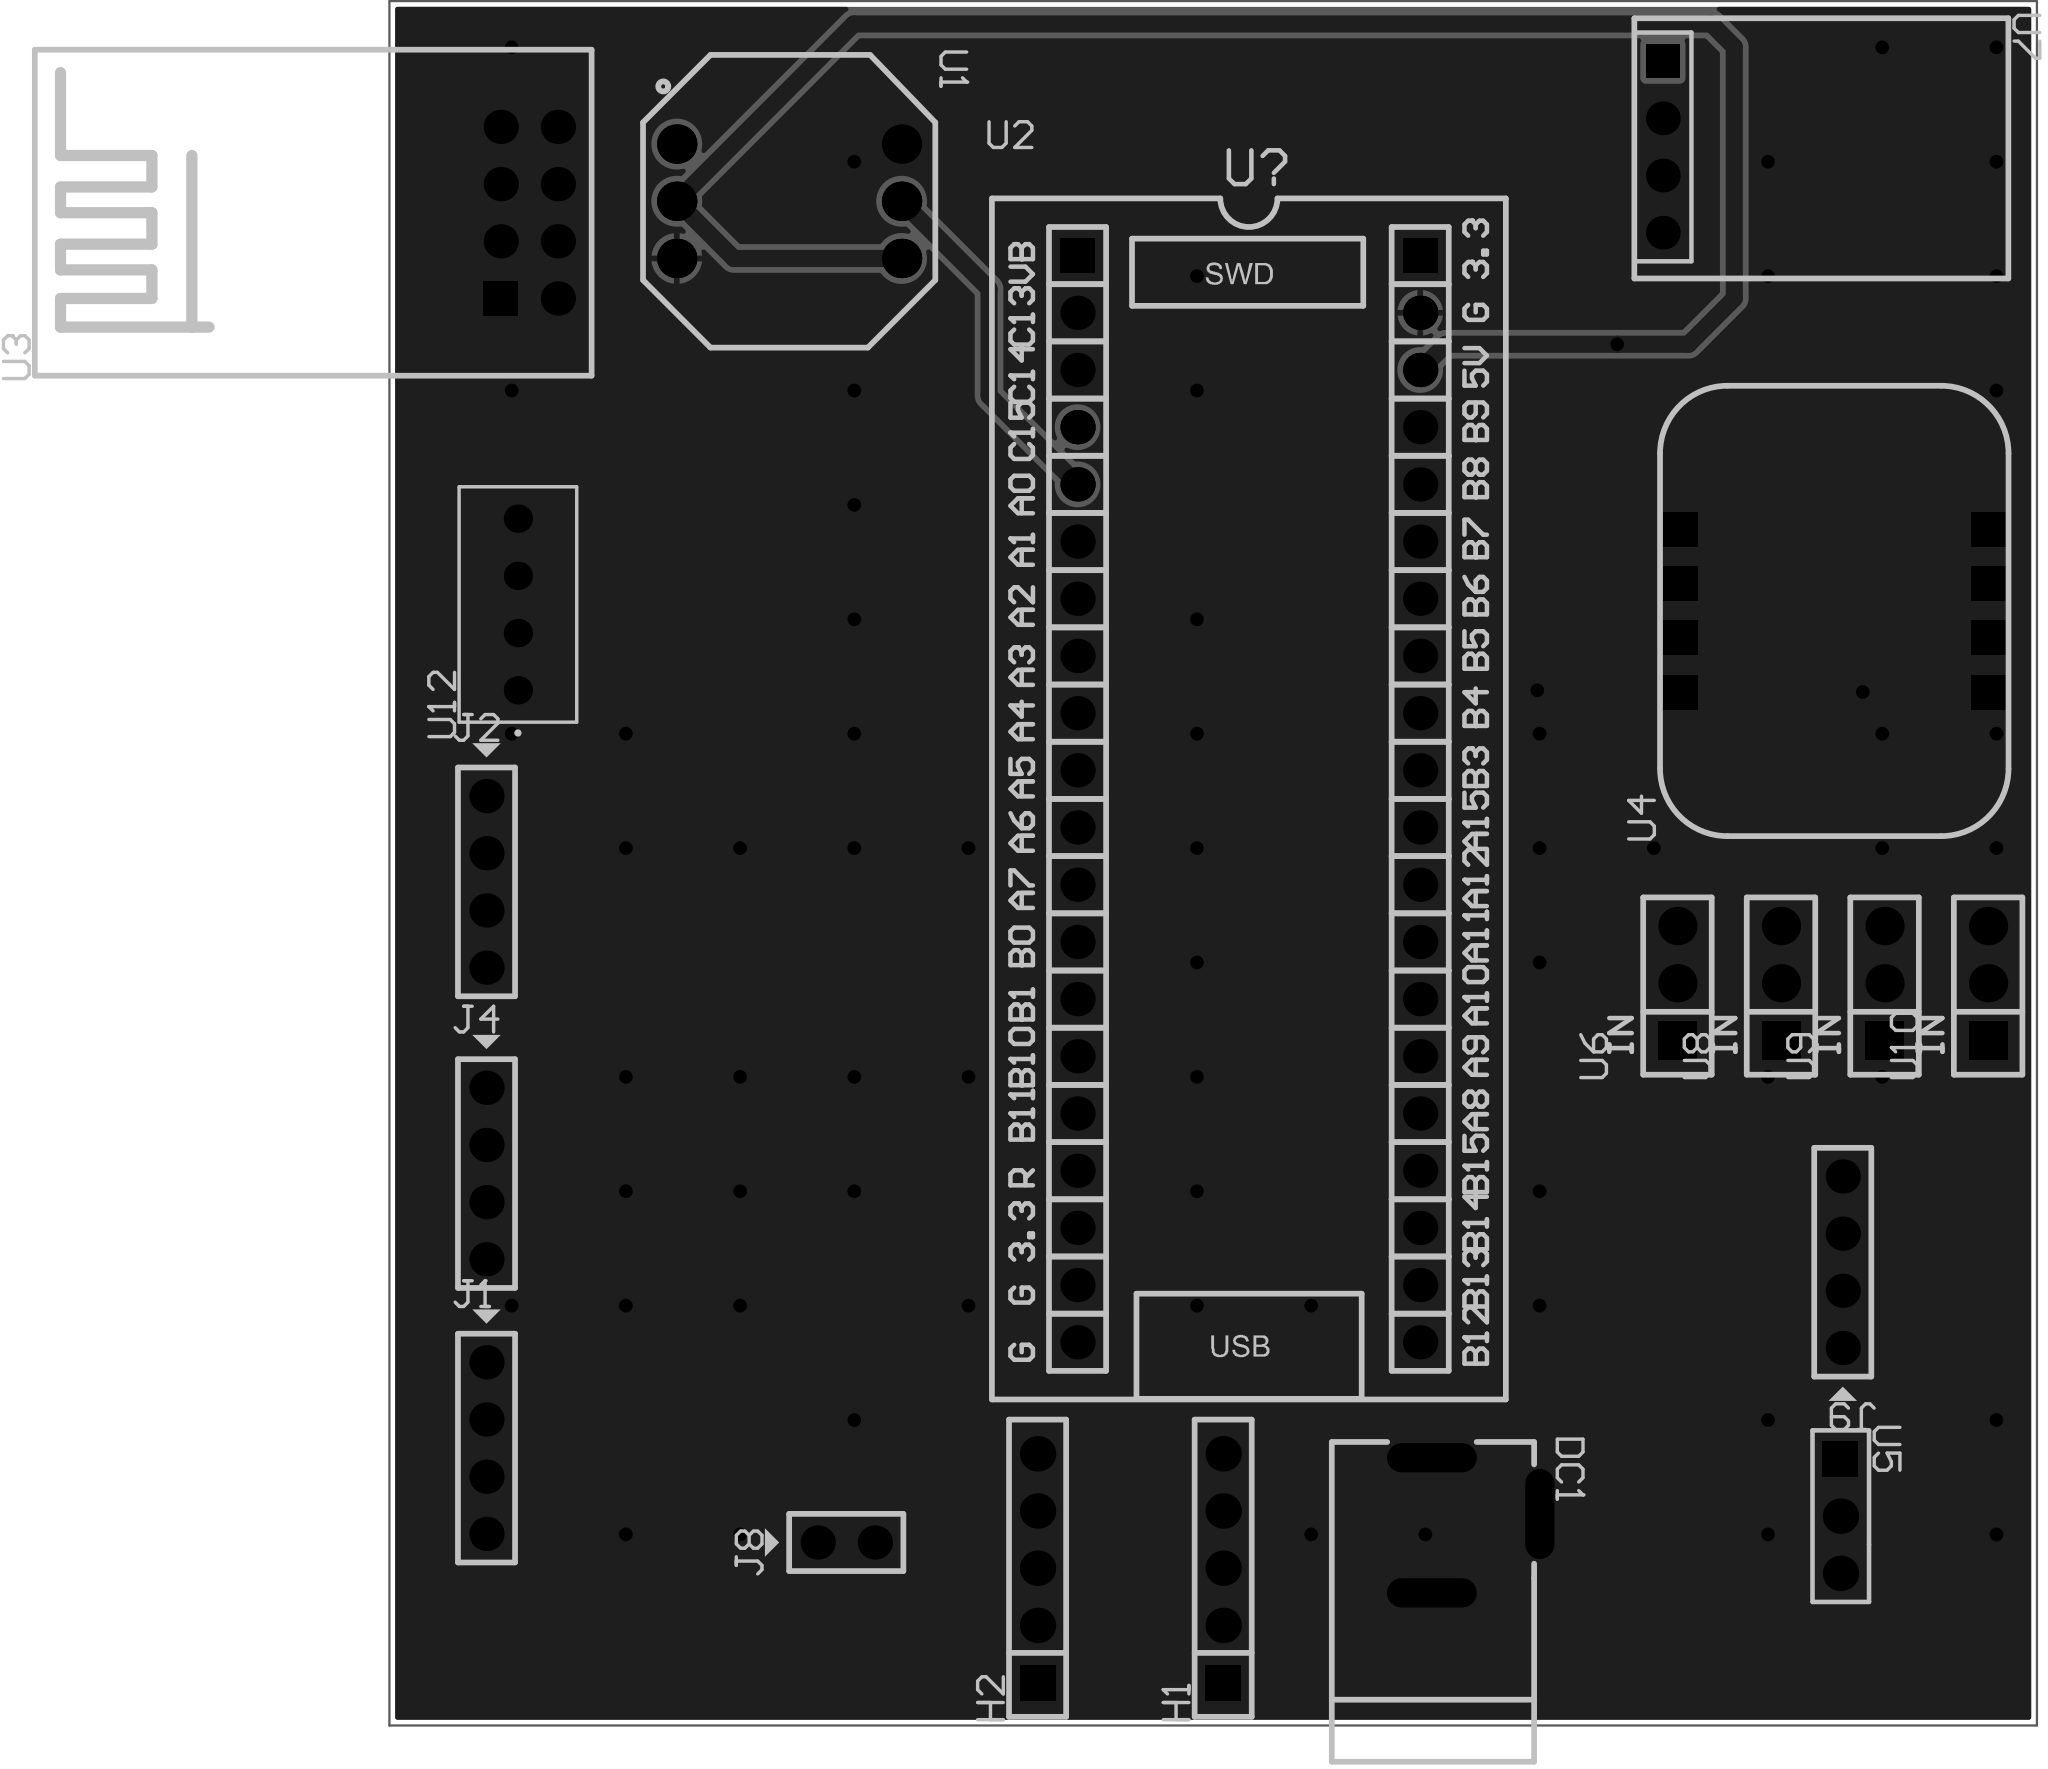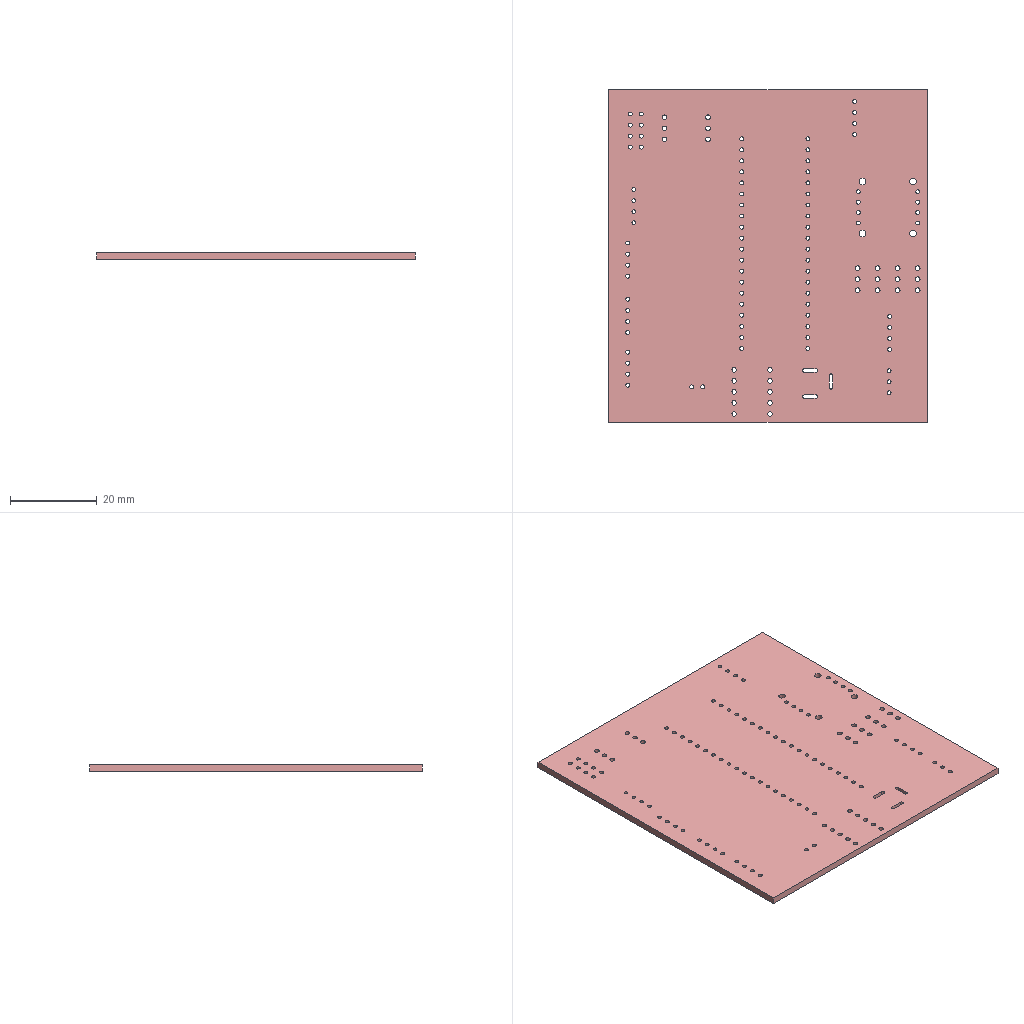Circuit board layout | Altium Designer | box 73.3 x 76.6 x 1.6 mm
Layer stack:
# Altium Designer layer stack of  (unit mm; dielectric type: 0 none, 1 core, 2 prepreg, 3 surface material)
index,name,kind,layer,copper_thickness_mm,dielectric_type,dielectric_thickness_mm,dielectric_material,dielectric_constant
0,Top Paste Mask Layer,other,,,,,,
1,Top Silkscreen Layer,other,,,,,,
2,Top Solder Mask Layer,dielectric,,,3,0.01,,3.3
3,Top Layer,copper,Top Layer,0.035,,,,
4,Dielectric1,dielectric,,,3,1.51,FR4,4.5
5,Bottom Layer,copper,Bottom Layer,0.035,,,,
6,Bottom Solder Mask Layer,dielectric,,,3,0.01,,3.3
7,Bottom Silkscreen Layer,other,,,,,,
8,Bottom Paste Mask Layer,other,,,,,,
# drill layer pairs: low layer,high layer
drill_pair,Top Layer,Bottom Layer
Part placement:
Designator,Comment,Layer,Footprint,Center-X(mm),Center-Y(mm),Rotation
J1,HDR-TH_4P-2.54MM,TopLayer,HDR-TH_4P-2.54MM,96.29,95.377,0
J2,HDR-TH_4P-2.54MM,TopLayer,HDR-TH_4P-2.54MM,96.29,120.523,0
J4,HDR-TH_4P-2.54MM,TopLayer,HDR-TH_4P-2.54MM,96.29,107.569,0
J8,HDR-TH_2P-2.54MM,TopLayer,HDR-TH_2P-2.54MM,112.292,91.186,90
J9,HDR-TH_4P-2.54MM,TopLayer,HDR-TH_4P-2.54MM,156.615,103.632,180
U1,XGZP6847A,TopLayer,SENSOR-TH_XGZP6847A,109.752,150.749,270
U2,STM32C8T6 minimum system,TopLayer,STM32F103C8T6最小系统插座,130.199,124.206,0
U3,ESP8266-01S,TopLayer,WIFIM-TH_ESP8266-01S,98.195,150.241,90
U4,MAX30102,TopLayer,MAX30102,156.234,132.555,90
U5,MH-FMD,TopLayer,MH-FMD,156.513,92.354,270
U6,SG90 servo - back (0-90),TopLayer,SG90,149.261,116.022,90
U7,GY-906-DCC,TopLayer,GY-906-DCC,148.614,153.162,270
U8,SG90 servo - leg (0-90),TopLayer,SG90,153.867,116.022,90
U9,SG90 servo - left flip (0-30),TopLayer,SG90,158.474,116.022,90
U10,SG90 servo - right flip (0-30),TopLayer,SG90,163.08,116.022,90
U12,,TopLayer,SHT30,97.687,132.842,90
DC1,,TopLayer,DC-2.0,140.74,91.948,270
H1,,TopLayer,HDR-TH_5P-P2.54-V-F,129.056,90.043,90
H2,,TopLayer,HDR-TH_5P-P2.54-V-F,120.801,90.043,90
Pad and via stacks:
# Altium Designer via and pad stacks of  (unit mm). Each distinct definition once, with the count of objects using it.
# via: kind,start_layer,end_layer,hole_mm,diameter_mm,mode(0 simple;1 top-mid-bottom;2 full stack),diameter_per_layer,count,example_net
# pad: kind,layer,hole_mm,hole_type(0 round;1 square;2 slot),plating,top_size,top_shape(1 round;2 rect;3 octagon;9 rounded rect),mid_size,bottom_size,mode,footprint,size_per_layer,count,example
pad,Multi-Layer,0.9144,0,plated,1.524x1.524,1,1.524x1.524,1.524x1.524,0,HDR-TH_4P-2.54MM,,16,J1.1
pad,Multi-Layer,0.9144,0,plated,1.524x1.524,1,1.524x1.524,1.524x1.524,0,HDR-TH_2P-2.54MM,,2,J8.1
pad,Multi-Layer,1.1,0,plated,1.75x1.75,1,1.75x1.75,1.75x1.75,0,SENSOR-TH_XGZP6847A,,6,U1.1
pad,Multi-Layer,0.9144,0,plated,1.524x1.524,2,1.524x1.524,1.524x1.524,0,STM32F103C8T6\u00D7\u00EE\u00D0\u00A1\u00CF\u00B5\u00CD\u00B3\u00B2\u00E5\u00D7\u00F9,,2,U2.40
pad,Multi-Layer,0.9144,0,plated,1.524x1.524,1,1.524x1.524,1.524x1.524,0,STM32F103C8T6\u00D7\u00EE\u00D0\u00A1\u00CF\u00B5\u00CD\u00B3\u00B2\u00E5\u00D7\u00F9,,38,U2.39
pad,Multi-Layer,0.9144,0,plated,1.524x1.524,1,1.524x1.524,1.524x1.524,0,WIFIM-TH_ESP8266-01S,,7,U3.8
pad,Multi-Layer,0.9144,0,plated,1.524x1.524,2,1.524x1.524,1.524x1.524,0,WIFIM-TH_ESP8266-01S,,1,U3.1
pad,Multi-Layer,0.9144,0,plated,1.524x1.524,2,1.524x1.524,1.524x1.524,0,MAX30102,,8,U4.1
pad,Multi-Layer,0.9144,0,plated,1.575x1.575,1,1.575x1.575,1.575x1.575,0,MH-FMD,,1,U5.3
pad,Multi-Layer,0.889,0,plated,1.575x1.575,1,1.575x1.575,1.575x1.575,0,MH-FMD,,1,U5.2
pad,Multi-Layer,0.889,0,plated,1.575x1.575,2,1.575x1.575,1.575x1.575,0,MH-FMD,,1,U5.1
pad,Multi-Layer,1.1,0,plated,1.7x1.7,2,1.7x1.7,1.7x1.7,0,SG90,,4,U6.1
pad,Multi-Layer,1.1,0,plated,1.7x1.7,1,1.7x1.7,1.7x1.7,0,SG90,,8,U6.2
pad,Multi-Layer,0.9,0,plated,1.5x1.5,1,1.5x1.5,1.5x1.5,0,GY-906-DCC,,3,U7.4
pad,Multi-Layer,0.9,0,plated,1.5x1.5,2,1.5x1.5,1.5x1.5,0,GY-906-DCC,,1,U7.1
pad,Multi-Layer,0.8401,0,plated,1.26x1.26,1,1.26x1.26,1.26x1.26,0,SHT30,,4,U12.1
pad,Multi-Layer,0.8001,2,plated,4x1.3,1,4x1.3,4x1.3,0,DC-2.0,,3,DC1.2
pad,Multi-Layer,1.02,0,plated,1.575x1.575,1,1.575x1.575,1.575x1.575,0,HDR-TH_5P-P2.54-V-F,,8,H1.5
pad,Multi-Layer,1.02,0,plated,1.575x1.575,2,1.575x1.575,1.575x1.575,0,HDR-TH_5P-P2.54-V-F,,2,H1.1
via,Top Layer,Bottom Layer,0.3048,0.61,0,,65,5V
Copper pours:
name,layer,net,type(0 solid;1 hatched;2 none)
Top Layer-GND,Top Layer,GND,0
Bottom Layer-GND,Bottom Layer,GND,0